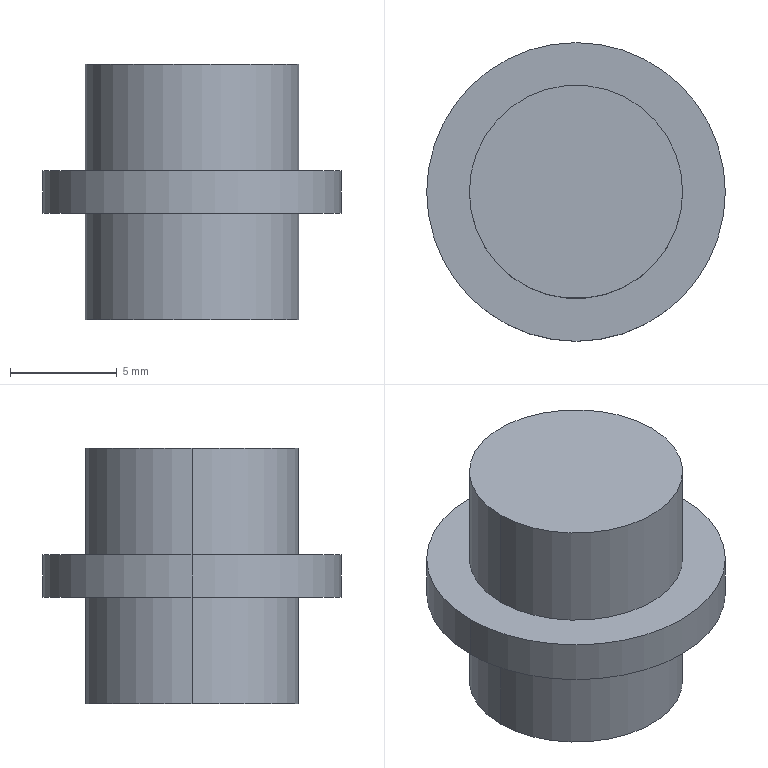Part | SolidWorks | features ICE 2, Extrusion 1 | 1 solid | 10 faces | box 14 x 14 x 12 mm | volume 1093 mm3 | cylinder 6 | plane 4 | commonest cylinder face diameters 10 x4 14 x2
STEP:
#1=CARTESIAN_POINT('',(5.,0.,12.));
#2=VERTEX_POINT('',#1);
#3=CARTESIAN_POINT('',(-5.,0.,12.));
#4=VERTEX_POINT('',#3);
#5=CARTESIAN_POINT('',(0.,0.,12.));
#6=DIRECTION('',(0.,0.,1.));
#7=DIRECTION('',(1.,0.,0.));
#8=AXIS2_PLACEMENT_3D('',#5,#6,#7);
#9=CIRCLE('',#8,5.);
#10=EDGE_CURVE('',#2,#4,#9,.T.);
#11=ORIENTED_EDGE('',*,*,#10,.F.);
#12=CARTESIAN_POINT('',(5.,0.,7.));
#13=VERTEX_POINT('',#12);
#14=CARTESIAN_POINT('',(5.,0.,12.));
#15=DIRECTION('',(0.,0.,-1.));
#16=VECTOR('',#15,1000.);
#17=LINE('',#14,#16);
#18=EDGE_CURVE('',#2,#13,#17,.T.);
#19=ORIENTED_EDGE('',*,*,#18,.T.);
#20=CARTESIAN_POINT('',(-5.,0.,7.));
#21=VERTEX_POINT('',#20);
#22=CARTESIAN_POINT('',(0.,0.,7.));
#23=DIRECTION('',(0.,0.,1.));
#24=DIRECTION('',(1.,0.,0.));
#25=AXIS2_PLACEMENT_3D('',#22,#23,#24);
#26=CIRCLE('',#25,5.);
#27=EDGE_CURVE('',#13,#21,#26,.T.);
#28=ORIENTED_EDGE('',*,*,#27,.T.);
#29=CARTESIAN_POINT('',(-5.,0.,12.));
#30=DIRECTION('',(0.,0.,-1.));
#31=VECTOR('',#30,1000.);
#32=LINE('',#29,#31);
#33=EDGE_CURVE('',#4,#21,#32,.T.);
#34=ORIENTED_EDGE('',*,*,#33,.F.);
#35=EDGE_LOOP('',(#11,#19,#28,#34));
#36=FACE_OUTER_BOUND('',#35,.T.);
#37=CARTESIAN_POINT('',(0.,0.,12.));
#38=DIRECTION('',(0.,0.,-1.));
#39=DIRECTION('',(-1.,0.,0.));
#40=AXIS2_PLACEMENT_3D('',#37,#38,#39);
#41=CYLINDRICAL_SURFACE('',#40,5.);
#42=ADVANCED_FACE('',(#36),#41,.T.);
#43=CARTESIAN_POINT('',(7.,0.,7.));
#44=VERTEX_POINT('',#43);
#45=CARTESIAN_POINT('',(-7.,0.,7.));
#46=VERTEX_POINT('',#45);
#47=CARTESIAN_POINT('',(0.,0.,7.));
#48=DIRECTION('',(0.,0.,1.));
#49=DIRECTION('',(1.,0.,0.));
#50=AXIS2_PLACEMENT_3D('',#47,#48,#49);
#51=CIRCLE('',#50,7.);
#52=EDGE_CURVE('',#44,#46,#51,.T.);
#53=ORIENTED_EDGE('',*,*,#52,.F.);
#54=CARTESIAN_POINT('',(7.,0.,5.));
#55=VERTEX_POINT('',#54);
#56=CARTESIAN_POINT('',(7.,0.,7.));
#57=DIRECTION('',(0.,0.,-1.));
#58=VECTOR('',#57,1000.);
#59=LINE('',#56,#58);
#60=EDGE_CURVE('',#44,#55,#59,.T.);
#61=ORIENTED_EDGE('',*,*,#60,.T.);
#62=CARTESIAN_POINT('',(-7.,0.,5.));
#63=VERTEX_POINT('',#62);
#64=CARTESIAN_POINT('',(0.,0.,5.));
#65=DIRECTION('',(0.,0.,1.));
#66=DIRECTION('',(1.,0.,0.));
#67=AXIS2_PLACEMENT_3D('',#64,#65,#66);
#68=CIRCLE('',#67,7.);
#69=EDGE_CURVE('',#55,#63,#68,.T.);
#70=ORIENTED_EDGE('',*,*,#69,.T.);
#71=CARTESIAN_POINT('',(-7.,0.,7.));
#72=DIRECTION('',(0.,0.,-1.));
#73=VECTOR('',#72,1000.);
#74=LINE('',#71,#73);
#75=EDGE_CURVE('',#46,#63,#74,.T.);
#76=ORIENTED_EDGE('',*,*,#75,.F.);
#77=EDGE_LOOP('',(#53,#61,#70,#76));
#78=FACE_OUTER_BOUND('',#77,.T.);
#79=CARTESIAN_POINT('',(0.,0.,7.));
#80=DIRECTION('',(0.,0.,-1.));
#81=DIRECTION('',(-1.,0.,0.));
#82=AXIS2_PLACEMENT_3D('',#79,#80,#81);
#83=CYLINDRICAL_SURFACE('',#82,7.);
#84=ADVANCED_FACE('',(#78),#83,.T.);
#85=CARTESIAN_POINT('',(5.,0.,5.));
#86=VERTEX_POINT('',#85);
#87=CARTESIAN_POINT('',(-5.,0.,5.));
#88=VERTEX_POINT('',#87);
#89=CARTESIAN_POINT('',(0.,0.,5.));
#90=DIRECTION('',(0.,0.,1.));
#91=DIRECTION('',(1.,0.,0.));
#92=AXIS2_PLACEMENT_3D('',#89,#90,#91);
#93=CIRCLE('',#92,5.);
#94=EDGE_CURVE('',#86,#88,#93,.T.);
#95=ORIENTED_EDGE('',*,*,#94,.F.);
#96=CARTESIAN_POINT('',(5.,0.,0.));
#97=VERTEX_POINT('',#96);
#98=CARTESIAN_POINT('',(5.,0.,5.));
#99=DIRECTION('',(0.,0.,-1.));
#100=VECTOR('',#99,1000.);
#101=LINE('',#98,#100);
#102=EDGE_CURVE('',#86,#97,#101,.T.);
#103=ORIENTED_EDGE('',*,*,#102,.T.);
#104=CARTESIAN_POINT('',(-5.,0.,0.));
#105=VERTEX_POINT('',#104);
#106=CARTESIAN_POINT('',(0.,0.,0.));
#107=DIRECTION('',(0.,0.,1.));
#108=DIRECTION('',(1.,0.,0.));
#109=AXIS2_PLACEMENT_3D('',#106,#107,#108);
#110=CIRCLE('',#109,5.);
#111=EDGE_CURVE('',#97,#105,#110,.T.);
#112=ORIENTED_EDGE('',*,*,#111,.T.);
#113=CARTESIAN_POINT('',(-5.,0.,5.));
#114=DIRECTION('',(0.,0.,-1.));
#115=VECTOR('',#114,1000.);
#116=LINE('',#113,#115);
#117=EDGE_CURVE('',#88,#105,#116,.T.);
#118=ORIENTED_EDGE('',*,*,#117,.F.);
#119=EDGE_LOOP('',(#95,#103,#112,#118));
#120=FACE_OUTER_BOUND('',#119,.T.);
#121=CARTESIAN_POINT('',(0.,0.,5.));
#122=DIRECTION('',(0.,0.,-1.));
#123=DIRECTION('',(-1.,0.,0.));
#124=AXIS2_PLACEMENT_3D('',#121,#122,#123);
#125=CYLINDRICAL_SURFACE('',#124,5.);
#126=ADVANCED_FACE('',(#120),#125,.T.);
#127=ORIENTED_EDGE('',*,*,#102,.F.);
#128=CARTESIAN_POINT('',(0.,0.,5.));
#129=DIRECTION('',(0.,0.,1.));
#130=DIRECTION('',(1.,0.,0.));
#131=AXIS2_PLACEMENT_3D('',#128,#129,#130);
#132=CIRCLE('',#131,5.);
#133=EDGE_CURVE('',#88,#86,#132,.T.);
#134=ORIENTED_EDGE('',*,*,#133,.F.);
#135=ORIENTED_EDGE('',*,*,#117,.T.);
#136=CARTESIAN_POINT('',(0.,0.,0.));
#137=DIRECTION('',(0.,0.,1.));
#138=DIRECTION('',(1.,0.,0.));
#139=AXIS2_PLACEMENT_3D('',#136,#137,#138);
#140=CIRCLE('',#139,5.);
#141=EDGE_CURVE('',#105,#97,#140,.T.);
#142=ORIENTED_EDGE('',*,*,#141,.T.);
#143=EDGE_LOOP('',(#127,#134,#135,#142));
#144=FACE_OUTER_BOUND('',#143,.T.);
#145=CARTESIAN_POINT('',(0.,0.,5.));
#146=DIRECTION('',(0.,0.,-1.));
#147=DIRECTION('',(-1.,0.,0.));
#148=AXIS2_PLACEMENT_3D('',#145,#146,#147);
#149=CYLINDRICAL_SURFACE('',#148,5.);
#150=ADVANCED_FACE('',(#144),#149,.T.);
#151=ORIENTED_EDGE('',*,*,#141,.F.);
#152=ORIENTED_EDGE('',*,*,#111,.F.);
#153=EDGE_LOOP('',(#151,#152));
#154=FACE_OUTER_BOUND('',#153,.T.);
#155=CARTESIAN_POINT('',(0.,0.,0.));
#156=DIRECTION('',(0.,0.,1.));
#157=DIRECTION('',(1.,0.,0.));
#158=AXIS2_PLACEMENT_3D('',#155,#156,#157);
#159=PLANE('',#158);
#160=ADVANCED_FACE('',(#154),#159,.F.);
#161=ORIENTED_EDGE('',*,*,#60,.F.);
#162=CARTESIAN_POINT('',(0.,0.,7.));
#163=DIRECTION('',(0.,0.,1.));
#164=DIRECTION('',(1.,0.,0.));
#165=AXIS2_PLACEMENT_3D('',#162,#163,#164);
#166=CIRCLE('',#165,7.);
#167=EDGE_CURVE('',#46,#44,#166,.T.);
#168=ORIENTED_EDGE('',*,*,#167,.F.);
#169=ORIENTED_EDGE('',*,*,#75,.T.);
#170=CARTESIAN_POINT('',(0.,0.,5.));
#171=DIRECTION('',(0.,0.,1.));
#172=DIRECTION('',(1.,0.,0.));
#173=AXIS2_PLACEMENT_3D('',#170,#171,#172);
#174=CIRCLE('',#173,7.);
#175=EDGE_CURVE('',#63,#55,#174,.T.);
#176=ORIENTED_EDGE('',*,*,#175,.T.);
#177=EDGE_LOOP('',(#161,#168,#169,#176));
#178=FACE_OUTER_BOUND('',#177,.T.);
#179=CARTESIAN_POINT('',(0.,0.,7.));
#180=DIRECTION('',(0.,0.,-1.));
#181=DIRECTION('',(-1.,0.,0.));
#182=AXIS2_PLACEMENT_3D('',#179,#180,#181);
#183=CYLINDRICAL_SURFACE('',#182,7.);
#184=ADVANCED_FACE('',(#178),#183,.T.);
#185=CARTESIAN_POINT('',(0.,0.,7.));
#186=DIRECTION('',(0.,0.,1.));
#187=DIRECTION('',(1.,0.,0.));
#188=AXIS2_PLACEMENT_3D('',#185,#186,#187);
#189=CIRCLE('',#188,5.);
#190=EDGE_CURVE('',#21,#13,#189,.T.);
#191=ORIENTED_EDGE('',*,*,#190,.F.);
#192=ORIENTED_EDGE('',*,*,#27,.F.);
#193=EDGE_LOOP('',(#191,#192));
#194=FACE_BOUND('',#193,.T.);
#195=ORIENTED_EDGE('',*,*,#167,.T.);
#196=ORIENTED_EDGE('',*,*,#52,.T.);
#197=EDGE_LOOP('',(#195,#196));
#198=FACE_OUTER_BOUND('',#197,.T.);
#199=CARTESIAN_POINT('',(0.,0.,7.));
#200=DIRECTION('',(0.,0.,1.));
#201=DIRECTION('',(1.,0.,0.));
#202=AXIS2_PLACEMENT_3D('',#199,#200,#201);
#203=PLANE('',#202);
#204=ADVANCED_FACE('',(#194,#198),#203,.T.);
#205=ORIENTED_EDGE('',*,*,#133,.T.);
#206=ORIENTED_EDGE('',*,*,#94,.T.);
#207=EDGE_LOOP('',(#205,#206));
#208=FACE_BOUND('',#207,.T.);
#209=ORIENTED_EDGE('',*,*,#175,.F.);
#210=ORIENTED_EDGE('',*,*,#69,.F.);
#211=EDGE_LOOP('',(#209,#210));
#212=FACE_OUTER_BOUND('',#211,.T.);
#213=CARTESIAN_POINT('',(0.,0.,5.));
#214=DIRECTION('',(0.,0.,1.));
#215=DIRECTION('',(1.,0.,0.));
#216=AXIS2_PLACEMENT_3D('',#213,#214,#215);
#217=PLANE('',#216);
#218=ADVANCED_FACE('',(#208,#212),#217,.F.);
#219=ORIENTED_EDGE('',*,*,#18,.F.);
#220=CARTESIAN_POINT('',(0.,0.,12.));
#221=DIRECTION('',(0.,0.,1.));
#222=DIRECTION('',(1.,0.,0.));
#223=AXIS2_PLACEMENT_3D('',#220,#221,#222);
#224=CIRCLE('',#223,5.);
#225=EDGE_CURVE('',#4,#2,#224,.T.);
#226=ORIENTED_EDGE('',*,*,#225,.F.);
#227=ORIENTED_EDGE('',*,*,#33,.T.);
#228=ORIENTED_EDGE('',*,*,#190,.T.);
#229=EDGE_LOOP('',(#219,#226,#227,#228));
#230=FACE_OUTER_BOUND('',#229,.T.);
#231=CARTESIAN_POINT('',(0.,0.,12.));
#232=DIRECTION('',(0.,0.,-1.));
#233=DIRECTION('',(-1.,0.,0.));
#234=AXIS2_PLACEMENT_3D('',#231,#232,#233);
#235=CYLINDRICAL_SURFACE('',#234,5.);
#236=ADVANCED_FACE('',(#230),#235,.T.);
#237=ORIENTED_EDGE('',*,*,#225,.T.);
#238=ORIENTED_EDGE('',*,*,#10,.T.);
#239=EDGE_LOOP('',(#237,#238));
#240=FACE_OUTER_BOUND('',#239,.T.);
#241=CARTESIAN_POINT('',(0.,0.,12.));
#242=DIRECTION('',(0.,0.,1.));
#243=DIRECTION('',(1.,0.,0.));
#244=AXIS2_PLACEMENT_3D('',#241,#242,#243);
#245=PLANE('',#244);
#246=ADVANCED_FACE('',(#240),#245,.T.);
#247=CLOSED_SHELL('',(#42,#84,#126,#150,#160,#184,#204,#218,#236,#246));
#248=MANIFOLD_SOLID_BREP('',#247);
#249=CARTESIAN_POINT('',(0.,0.,0.));
#250=DIRECTION('',(0.,0.,1.));
#251=DIRECTION('',(1.,0.,0.));
#252=AXIS2_PLACEMENT_3D('',#249,#250,#251);
#253=(LENGTH_UNIT()NAMED_UNIT(*)SI_UNIT(.MILLI.,.METRE.));
#254=UNCERTAINTY_MEASURE_WITH_UNIT(LENGTH_MEASURE(0.00001),#253,'','');
#255=(NAMED_UNIT(*)PLANE_ANGLE_UNIT()SI_UNIT($,.RADIAN.));
#256=(NAMED_UNIT(*)SI_UNIT($,.STERADIAN.)SOLID_ANGLE_UNIT());
#257=(GEOMETRIC_REPRESENTATION_CONTEXT(3)GLOBAL_UNCERTAINTY_ASSIGNED_CONTEXT((#254))GLOBAL_UNIT_ASSIGNED_CONTEXT((#253,#255,#256))REPRESENTATION_CONTEXT('',''));
#258=ADVANCED_BREP_SHAPE_REPRESENTATION('',(#248,#252),#257);